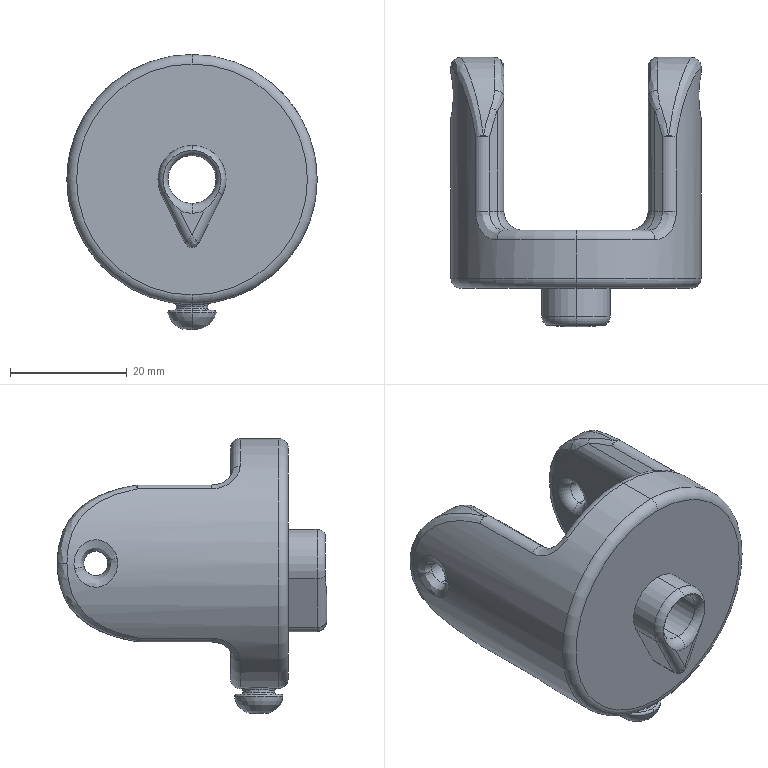Part | SolidWorks | features Fillet 11, ICE 9, Extrusion 1, Scale 1 | 1 solid | 104 faces | box 42.926 x 46.228 x 47.219 mm | volume 24971 mm3 | spline 31 | cylinder 31 | torus 25 | plane 13 | sphere 4 | commonest cylinder face diameters 6.604 x10 3.302 x8 4.194 x4 5.424 x2 8.255 x2 11.7 x2